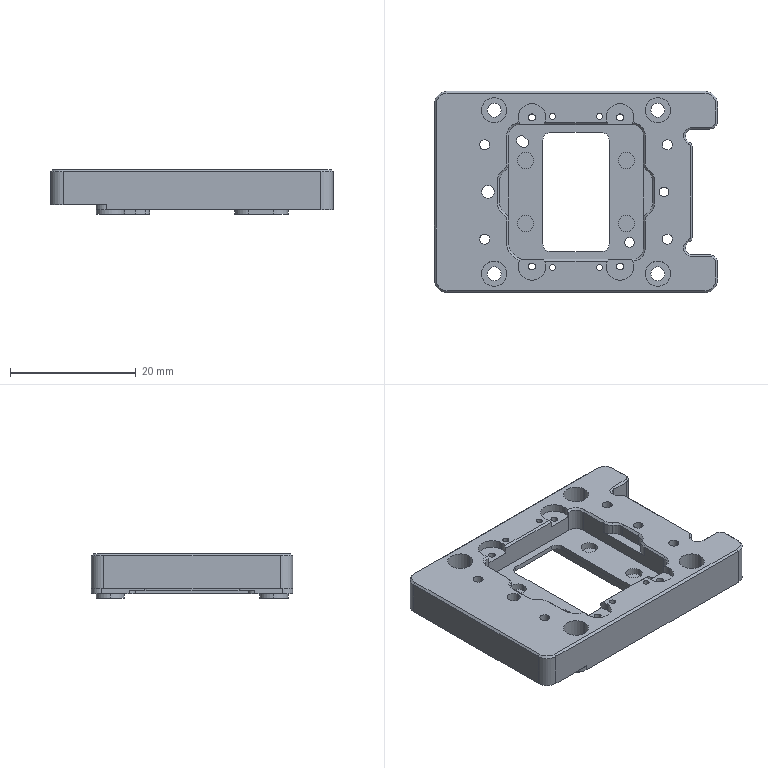NC program | NX | posted with a generic post | part box 45 x 32 x 7.05 mm
Lines 1284 to 2424 of 5787:
(CAVITY_MILL , TOOL : D3)
N2518 T17 M6
N2520 G54
N2522 G17 G0 G90 X-5.414 Y8.674 S9500 M3
N2524 G43 Z30. H17
N2526 Z0.75
N2528 G94 G1 Z-0.25 F1100.
N2530 G3 X-5.887 Y9.474 R1.
N2532 G2 X-6.394 Y11.499 R1.498
N2534 G3 X-7.606 Y11.5 R-0.7
N2536 G2 X-8.12 Y9.472 R1.505
N2538 G3 X-8.594 Y8.592 R1.
N2540 G1 X-8.563 Y7.553
N2542 Z0.75
N2544 G0 Z30.
N2546 X-5.938 Y8.753
N2548 Z0.75
N2550 G1 Z-0.25
N2552 X-7.156 Y9.453
N2554 G3 X-8.156 Y9.451 R1.
N2556 G2 X-9. Y9.25 R1.505
N2558 G3 X-9.25 Y9. R0.25
N2560 G1 Y7.912
N2562 G3 X-8.75 Y7.046 R1.
N2564 G1 X-8.65 Y6.988
N2566 Z0.75
N2568 G0 Z30.
N2570 X-5.417 Y8.6
N2572 Z0.5
N2574 G1 Z-0.5
N2576 G3 X-5.899 Y9.416 R1.
N2578 G2 X-6.403 Y11.484 R1.5
N2580 G3 X-7.7 Y11.835 R-0.7
N2582 X-7.581 Y11.458 R0.701
N2584 G2 X-8.101 Y9.416 R1.5
N2586 G3 X-7.722 Y9.742 R0.5
N2588 G1 X-7.646 Y8.644
N2590 Z0.5
N2592 G0 Z30.
N2594 X-5.417 Y8.6
N2596 Z0.25
N2598 G1 Z-0.75
N2600 G3 X-5.899 Y9.416 R1.
N2602 G2 X-6.403 Y11.484 R1.5
N2604 G3 X-7.7 Y11.835 R-0.7
N2606 X-7.581 Y11.458 R0.701
N2608 G2 X-8.101 Y9.416 R1.5
N2610 G3 X-7.722 Y9.742 R0.5
N2612 G1 X-7.646 Y8.644
N2614 Z0.25
N2616 G0 Z30.
N2618 X-5.417 Y8.6
N2620 Z0.
N2622 G1 Z-1.
N2624 G3 X-5.899 Y9.416 R1.
N2626 G2 X-6.528 Y11.229 R1.5
N2628 X-6.388 Y11.51 R1.501
N2630 G3 X-7.597 Y11.484 R-0.7
N2632 G2 X-8.101 Y9.416 R1.5
N2634 G3 X-7.722 Y9.742 R0.5
N2636 G1 X-7.213 Y8.766
N2638 Z0.
N2640 G0 X-5.417 Y8.6 Z-0.25
N2642 G1 Z-1.25
N2644 G3 X-5.899 Y9.416 R1.
N2646 G2 X-6.528 Y11.229 R1.5
N2648 X-6.388 Y11.51 R1.501
N2650 G3 X-7.7 Y11.835 R-0.7
N2652 X-7.592 Y11.477 R0.7
N2654 G2 X-8.101 Y9.416 R1.5
N2656 G3 X-7.722 Y9.742 R0.5
N2658 G1 X-7.213 Y8.766
N2660 Z-0.25
N2662 G0 Z30.
N2664 X-1.255 Y7.4
N2666 Z-3.113
N2668 G1 Z-4.113
N2670 X-1.312 Y7.5
N2672 G3 X-2.178 Y8. R1.
N2674 G1 X-3.75
N2676 Y6.428
N2678 G3 X-3.25 Y5.562 R1.
N2680 G1 X-3.15 Y5.505
N2682 Z-3.113
N2684 G0 X-1.255 Y7.4 Z-3.375
N2686 G1 Z-4.375
N2688 X-1.312 Y7.5
N2690 G3 X-2.178 Y8. R1.
N2692 G1 X-3.75
N2694 Y6.428
N2696 G3 X-3.25 Y5.562 R1.
N2698 G1 X-3.15 Y5.505
N2700 Z-3.375
N2702 G0 X-1.256 Y7.4 Z-3.638
N2704 G1 Z-4.638
N2706 X-1.314 Y7.5
N2708 G3 X-2.18 Y8. R1.
N2710 G1 X-3.75
N2712 Y6.43
N2714 G3 X-3.25 Y5.564 R1.
N2716 G1 X-3.15 Y5.506
N2718 Z-3.638
N2720 G0 X-1.256 Y7.4 Z-3.9
N2722 G1 Z-4.9
N2724 X-1.314 Y7.5
N2726 G3 X-2.18 Y8. R1.
N2728 G1 X-3.75
N2730 Y6.43
N2732 G3 X-3.25 Y5.564 R1.
N2734 G1 X-3.15 Y5.506
N2736 Z-3.9
N2738 G0 X-1.256 Y7.4 Z-4.169
N2740 G1 Z-5.169
N2742 X-1.314 Y7.5
N2744 G3 X-2.18 Y8. R1.
N2746 G1 X-3.75
N2748 Y6.43
N2750 G3 X-3.25 Y5.564 R1.
N2752 G1 X-3.15 Y5.506
N2754 Z-4.169
N2756 G0 X-1.256 Y7.4 Z-4.438
N2758 G1 Z-5.438
N2760 X-1.314 Y7.5
N2762 G3 X-2.18 Y8. R1.
N2764 G1 X-3.75
N2766 Y6.43
N2768 G3 X-3.25 Y5.564 R1.
N2770 G1 X-3.15 Y5.506
N2772 Z-4.438
N2774 G0 X-1.256 Y7.4 Z-4.706
N2776 G1 Z-5.706
N2778 X-1.314 Y7.5
N2780 G3 X-2.18 Y8. R1.
N2782 G1 X-3.75
N2784 Y6.43
N2786 G3 X-3.25 Y5.564 R1.
N2788 G1 X-3.15 Y5.506
N2790 Z-4.706
N2792 G0 X-1.256 Y7.4 Z-4.975
N2794 G1 Z-5.975
N2796 X-1.314 Y7.5
N2798 G3 X-2.18 Y8. R1.
N2800 G1 X-3.75
N2802 Y6.43
N2804 G3 X-3.25 Y5.564 R1.
N2806 G1 X-3.15 Y5.506
N2808 Z-4.975
N2810 G0 X-1.256 Y7.4 Z-5.244
N2812 G1 Z-6.244
N2814 X-1.314 Y7.5
N2816 G3 X-2.18 Y8. R1.
N2818 G1 X-3.75
N2820 Y6.43
N2822 G3 X-3.25 Y5.564 R1.
N2824 G1 X-3.15 Y5.506
N2826 Z-5.244
N2828 G0 X-1.256 Y7.4 Z-5.513
N2830 G1 Z-6.513
N2832 X-1.314 Y7.5
N2834 G3 X-2.18 Y8. R1.
N2836 G1 X-3.75
N2838 Y6.43
N2840 G3 X-3.25 Y5.564 R1.
N2842 G1 X-3.15 Y5.506
N2844 Z-5.513
N2846 G0 X-1.256 Y7.4 Z-5.781
N2848 G1 Z-6.781
N2850 X-1.314 Y7.5
N2852 G3 X-2.18 Y8. R1.
N2854 G1 X-3.75
N2856 Y6.43
N2858 G3 X-3.25 Y5.564 R1.
N2860 G1 X-3.15 Y5.506
N2862 Z-5.781
N2864 G0 X-1.256 Y7.4 Z-6.05
N2866 G1 Z-7.05
N2868 X-1.314 Y7.5
N2870 G3 X-2.18 Y8. R1.
N2872 G1 X-3.75
N2874 Y6.43
N2876 G3 X-3.25 Y5.564 R1.
N2878 G1 X-3.15 Y5.506
N2880 Z-6.05
N2882 G0 Z30.
N2884 X-5.649 Y8.6
N2886 Z0.5
N2888 G1 Z-0.5
N2890 X-7.111 Y9.421
N2892 G3 X-8.111 Y9.41 R1.
N2894 G2 X-8.876 Y9.2 R1.5
N2896 G1 X-9.
N2898 G3 X-9.2 Y9. R0.2
N2900 G1 Y7.868
N2902 G3 X-8.7 Y7.002 R1.
N2904 G1 X-8.6 Y6.945
N2906 Z0.5
N2908 G0 Z30.
N2910 X-5.649 Y8.6
N2912 Z0.25
N2914 G1 Z-0.75
N2916 X-7.111 Y9.421
N2918 G3 X-8.111 Y9.41 R1.
N2920 G2 X-8.876 Y9.2 R1.5
N2922 G1 X-9.
N2924 G3 X-9.2 Y9. R0.2
N2926 G1 Y7.868
N2928 G3 X-8.7 Y7.002 R1.
N2930 G1 X-8.6 Y6.945
N2932 Z0.25
N2934 G0 Z30.
N2936 X-5.649 Y8.6
N2938 Z0.
N2940 G1 Z-1.
N2942 X-7.111 Y9.421
N2944 G3 X-8.111 Y9.41 R1.
N2946 G2 X-8.876 Y9.2 R1.5
N2948 G1 X-9.
N2950 G3 X-9.2 Y9. R0.2
N2952 G1 Y7.868
N2954 G3 X-8.7 Y7.002 R1.
N2956 G1 X-8.6 Y6.945
N2958 Z0.
N2960 G0 X-5.649 Y8.6 Z-0.25
N2962 G1 Z-1.25
N2964 X-7.111 Y9.421
N2966 G3 X-8.111 Y9.41 R1.
N2968 G2 X-8.876 Y9.2 R1.5
N2970 G1 X-9.
N2972 G3 X-9.2 Y9. R0.2
N2974 G1 Y7.868
N2976 G3 X-8.7 Y7.002 R1.
N2978 G1 X-8.6 Y6.945
N2980 Z-0.25
N2982 G0 X-6.705 Y8.6 Z-0.5
N2984 G1 Z-1.5
N2986 X-6.762 Y8.7
N2988 G3 X-7.628 Y9.2 R1.
N2990 G1 X-9.
N2992 G3 X-9.2 Y9. R0.2
N2994 G1 Y7.628
N2996 G3 X-8.7 Y6.762 R1.
N2998 G1 X-8.6 Y6.705
N3000 Z-0.5
N3002 G0 X-6.705 Y8.6 Z-0.75
N3004 G1 Z-1.75
N3006 X-6.762 Y8.7
N3008 G3 X-7.628 Y9.2 R1.
N3010 G1 X-9.
N3012 G3 X-9.2 Y9. R0.2
N3014 G1 Y7.628
N3016 G3 X-8.7 Y6.762 R1.
N3018 G1 X-8.6 Y6.705
N3020 Z-0.75
N3022 G0 X-6.705 Y8.6 Z-1.
N3024 G1 Z-2.
N3026 X-6.762 Y8.7
N3028 G3 X-7.628 Y9.2 R1.
N3030 G1 X-9.
N3032 G3 X-9.2 Y9. R0.2
N3034 G1 Y7.628
N3036 G3 X-8.7 Y6.762 R1.
N3038 G1 X-8.6 Y6.705
N3040 Z-1.
N3042 G0 X-6.705 Y8.6 Z-1.25
N3044 G1 Z-2.25
N3046 X-6.762 Y8.7
N3048 G3 X-7.628 Y9.2 R1.
N3050 G1 X-9.
N3052 G3 X-9.2 Y9. R0.2
N3054 G1 Y7.628
N3056 G3 X-8.7 Y6.762 R1.
N3058 G1 X-8.6 Y6.705
N3060 Z-1.25
N3062 G0 X-6.705 Y8.6 Z-1.5
N3064 G1 Z-2.5
N3066 X-6.762 Y8.7
N3068 G3 X-7.628 Y9.2 R1.
N3070 G1 X-9.
N3072 G3 X-9.2 Y9. R0.2
N3074 G1 Y7.628
N3076 G3 X-8.7 Y6.762 R1.
N3078 G1 X-8.6 Y6.705
N3080 Z-1.5
N3082 G0 X-6.705 Y8.6 Z-1.75
N3084 G1 Z-2.75
N3086 X-6.762 Y8.7
N3088 G3 X-7.628 Y9.2 R1.
N3090 G1 X-9.
N3092 G3 X-9.2 Y9. R0.2
N3094 G1 Y7.628
N3096 G3 X-8.7 Y6.762 R1.
N3098 G1 X-8.6 Y6.705
N3100 Z-1.75
N3102 G0 X-6.705 Y8.6 Z-2.
N3104 G1 Z-3.
N3106 X-6.762 Y8.7
N3108 G3 X-7.628 Y9.2 R1.
N3110 G1 X-9.
N3112 G3 X-9.2 Y9. R0.2
N3114 G1 Y7.628
N3116 G3 X-8.7 Y6.762 R1.
N3118 G1 X-8.6 Y6.705
N3120 Z-2.
N3122 G0 X-6.705 Y8.6 Z-2.283
N3124 G1 Z-3.283
N3126 X-6.762 Y8.7
N3128 G3 X-7.628 Y9.2 R1.
N3130 G1 X-9.
N3132 G3 X-9.2 Y9. R0.2
N3134 G1 Y7.628
N3136 G3 X-8.7 Y6.762 R1.
N3138 G1 X-8.6 Y6.705
N3140 Z-2.283
N3142 G0 X-6.705 Y8.6 Z-2.567
N3144 G1 Z-3.567
N3146 X-6.762 Y8.7
N3148 G3 X-7.628 Y9.2 R1.
N3150 G1 X-9.
N3152 G3 X-9.2 Y9. R0.2
N3154 G1 Y7.628
N3156 G3 X-8.7 Y6.762 R1.
N3158 G1 X-8.6 Y6.705
N3160 Z-2.567
N3162 G0 X-6.705 Y8.6 Z-2.85
N3164 G1 Z-3.85
N3166 X-6.762 Y8.7
N3168 G3 X-7.628 Y9.2 R1.
N3170 G1 X-9.
N3172 G3 X-9.2 Y9. R0.2
N3174 G1 Y7.628
N3176 G3 X-8.7 Y6.762 R1.
N3178 G1 X-8.6 Y6.705
N3180 Z-2.85
N3182 G0 Z30.
N3184 X-9.203 Y2.649
N3186 Z0.75
N3188 G1 Z-0.25
N3190 G3 X-10.166 Y2.381 R1.
N3192 G2 X-10.621 Y1.996 R3.2
N3194 G3 X-10.75 Y1.75 R0.3
N3196 G1 Y1.108
N3198 G3 X-10.25 Y0.242 R1.
N3200 G1 X-10.15 Y0.185
N3202 Z0.75
N3204 G0 Z30.
N3206 X-9.158 Y2.625
N3208 Z0.5
N3210 G1 X-9.16 Y2.626 Z-0.5
N3212 G3 X-10.122 Y2.354 R1.
N3214 G2 X-10.593 Y1.955 R3.25
N3216 G3 X-10.7 Y1.75 R0.25
N3218 G1 Y1.087
N3220 G3 X-10.2 Y0.221 R1.
N3222 G1 X-10.1 Y0.163
N3224 Z0.5
N3226 G0 Z30.
N3228 X-9.158 Y2.625
N3230 Z0.25
N3232 G1 X-9.16 Y2.626 Z-0.75
N3234 G3 X-10.122 Y2.354 R1.
N3236 G2 X-10.593 Y1.955 R3.25
N3238 G3 X-10.7 Y1.75 R0.25
N3240 G1 Y1.087
N3242 G3 X-10.2 Y0.221 R1.
N3244 G1 X-10.1 Y0.163
N3246 Z0.25
N3248 G0 Z30.
N3250 X-9.158 Y2.625
N3252 Z0.
N3254 G1 X-9.16 Y2.626 Z-1.
N3256 G3 X-10.122 Y2.354 R1.
N3258 G2 X-10.593 Y1.955 R3.25
N3260 G3 X-10.7 Y1.75 R0.25
N3262 G1 Y1.087
N3264 G3 X-10.2 Y0.221 R1.
N3266 G1 X-10.1 Y0.163
N3268 Z0.
N3270 G0 X-9.158 Y2.625 Z-0.25
N3272 G1 X-9.16 Y2.626 Z-1.25
N3274 G3 X-10.122 Y2.354 R1.
N3276 G2 X-10.593 Y1.955 R3.25
N3278 G3 X-10.7 Y1.75 R0.25
N3280 G1 Y1.087
N3282 G3 X-10.2 Y0.221 R1.
N3284 G1 X-10.1 Y0.163
N3286 Z-0.25
N3288 G0 X-9.158 Y2.625 Z-0.5
N3290 G1 X-9.16 Y2.626 Z-1.5
N3292 G3 X-10.122 Y2.354 R1.
N3294 G2 X-10.593 Y1.955 R3.25
N3296 G3 X-10.7 Y1.75 R0.25
N3298 G1 Y1.087
N3300 G3 X-10.2 Y0.221 R1.
N3302 G1 X-10.1 Y0.163
N3304 Z-0.5
N3306 G0 X-9.158 Y2.625 Z-0.75
N3308 G1 X-9.16 Y2.626 Z-1.75
N3310 G3 X-10.122 Y2.354 R1.
N3312 G2 X-10.593 Y1.955 R3.25
N3314 G3 X-10.7 Y1.75 R0.25
N3316 G1 Y1.087
N3318 G3 X-10.2 Y0.221 R1.
N3320 G1 X-10.1 Y0.163
N3322 Z-0.75
N3324 G0 X-9.158 Y2.625 Z-1.
N3326 G1 X-9.16 Y2.626 Z-2.
N3328 G3 X-10.122 Y2.354 R1.
N3330 G2 X-10.593 Y1.955 R3.25
N3332 G3 X-10.7 Y1.75 R0.25
N3334 G1 Y1.087
N3336 G3 X-10.2 Y0.221 R1.
N3338 G1 X-10.1 Y0.163
N3340 Z-1.
N3342 G0 Z30.
N3344 X-10.15 Y-0.185
N3346 Z0.75
N3348 G1 Z-0.25
N3350 X-10.25 Y-0.242
N3352 G3 X-10.75 Y-1.108 R1.
N3354 G1 Y-1.75
N3356 G3 X-10.621 Y-1.996 R0.3
N3358 G2 X-10.166 Y-2.381 R3.2
N3360 G3 X-9.203 Y-2.649 R1.
N3362 G1 Z0.75
N3364 G0 Z30.
N3366 X-10.1 Y-0.163
N3368 Z0.5
N3370 G1 Z-0.5
N3372 X-10.2 Y-0.221
N3374 G3 X-10.7 Y-1.087 R1.
N3376 G1 Y-1.75
N3378 G3 X-10.593 Y-1.955 R0.25
N3380 G2 X-10.122 Y-2.354 R3.25
N3382 G3 X-9.158 Y-2.625 R1.
N3384 G1 Z0.5
N3386 G0 Z30.
N3388 X-10.1 Y-0.163
N3390 Z0.25
N3392 G1 Z-0.75
N3394 X-10.2 Y-0.221
N3396 G3 X-10.7 Y-1.087 R1.
N3398 G1 Y-1.75
N3400 G3 X-10.593 Y-1.955 R0.25
N3402 G2 X-10.122 Y-2.354 R3.25
N3404 G3 X-9.158 Y-2.625 R1.
N3406 G1 Z0.25
N3408 G0 Z30.
N3410 X-10.1 Y-0.163
N3412 Z0.
N3414 G1 Z-1.
N3416 X-10.2 Y-0.221
N3418 G3 X-10.7 Y-1.087 R1.
N3420 G1 Y-1.75
N3422 G3 X-10.593 Y-1.955 R0.25
N3424 G2 X-10.122 Y-2.354 R3.25
N3426 G3 X-9.158 Y-2.625 R1.
N3428 G1 Z0.
N3430 G0 X-10.1 Y-0.163 Z-0.25
N3432 G1 Z-1.25
N3434 X-10.2 Y-0.221
N3436 G3 X-10.7 Y-1.087 R1.
N3438 G1 Y-1.75
N3440 G3 X-10.593 Y-1.955 R0.25
N3442 G2 X-10.122 Y-2.354 R3.25
N3444 G3 X-9.158 Y-2.625 R1.
N3446 G1 Z-0.25
N3448 G0 X-10.1 Y-0.163 Z-0.5
N3450 G1 Z-1.5
N3452 X-10.2 Y-0.221
N3454 G3 X-10.7 Y-1.087 R1.
N3456 G1 Y-1.75
N3458 G3 X-10.593 Y-1.955 R0.25
N3460 G2 X-10.122 Y-2.354 R3.25
N3462 G3 X-9.158 Y-2.625 R1.
N3464 G1 Z-0.5
N3466 G0 X-10.1 Y-0.163 Z-0.75
N3468 G1 Z-1.75
N3470 X-10.2 Y-0.221
N3472 G3 X-10.7 Y-1.087 R1.
N3474 G1 Y-1.75
N3476 G3 X-10.593 Y-1.955 R0.25
N3478 G2 X-10.122 Y-2.354 R3.25
N3480 G3 X-9.158 Y-2.625 R1.
N3482 G1 Z-0.75
N3484 G0 X-10.1 Y-0.163 Z-1.
N3486 G1 Z-2.
N3488 X-10.2 Y-0.221
N3490 G3 X-10.7 Y-1.087 R1.
N3492 G1 Y-1.75
N3494 G3 X-10.593 Y-1.955 R0.25
N3496 G2 X-10.122 Y-2.354 R3.25
N3498 G3 X-9.158 Y-2.625 R1.
N3500 G1 Z-1.
N3502 G0 Z30.
N3504 X-8.65 Y-6.866
N3506 Z0.75
N3508 G1 Z-0.25
N3510 X-8.75 Y-6.923
N3512 G3 X-9.25 Y-7.789 R1.
N3514 G1 Y-8.379
N3516 X-9.259 Y-8.486
N3518 X-9.177 Y-8.555
N3520 X-8.76 Y-8.972
N3522 G3 X-7.794 Y-9.231 R1.
N3524 G1 X-5.904 Y-8.725
N3526 Z0.75
N3528 G0 Z30.
N3530 X-8.6 Y-6.845
N3532 Z0.5
N3534 G1 Z-0.5
N3536 X-8.7 Y-6.903
N3538 G3 X-9.2 Y-7.769 R1.
N3540 G1 Y-8.379
N3542 X-9.212 Y-8.467
N3544 X-9.141 Y-8.52
N3546 X-8.71 Y-8.951
N3548 G3 X-8.227 Y-9.081 R0.5
N3550 G1 X-7.036 Y-8.762
N3552 Z0.5
N3554 G0 Z30.
N3556 X-8.6 Y-6.845
N3558 Z0.25
N3560 G1 Z-0.75
N3562 X-8.7 Y-6.903
N3564 G3 X-9.2 Y-7.769 R1.
N3566 G1 Y-8.379
N3568 X-9.212 Y-8.467
N3570 X-9.141 Y-8.52
N3572 X-8.71 Y-8.951
N3574 G3 X-8.227 Y-9.081 R0.5
N3576 G1 X-7.036 Y-8.762
N3578 Z0.25
N3580 G0 Z30.
N3582 X-8.6 Y-6.845
N3584 Z0.
N3586 G1 Z-1.
N3588 X-8.7 Y-6.903
N3590 G3 X-9.2 Y-7.769 R1.
N3592 G1 Y-8.379
N3594 X-9.212 Y-8.467
N3596 X-9.141 Y-8.52
N3598 X-8.71 Y-8.951
N3600 G3 X-8.227 Y-9.081 R0.5
N3602 G1 X-7.036 Y-8.762
N3604 Z0.
N3606 G0 X-8.6 Y-6.845 Z-0.25
N3608 G1 Z-1.25
N3610 X-8.7 Y-6.903
N3612 G3 X-9.2 Y-7.769 R1.
N3614 G1 Y-8.379
N3616 X-9.212 Y-8.467
N3618 X-9.141 Y-8.52
N3620 X-8.71 Y-8.951
N3622 G3 X-8.227 Y-9.081 R0.5
N3624 G1 X-7.036 Y-8.762
N3626 Z-0.25
N3628 G0 Z30.
N3630 X-8.485 Y-7.499
N3632 Z0.75
N3634 G1 Z-0.25
N3636 X-8.526 Y-8.528
N3638 G3 X-8.061 Y-9.414 R1.
N3640 G2 X-7.584 Y-11.464 R1.498
N3642 G3 X-6.394 Y-11.499 R-0.7
N3644 G2 X-5.852 Y-9.453 R1.498
N3646 G3 X-5.358 Y-8.666 R1.
N3648 G1 Z0.75
N3650 G0 Z30.
N3652 X-8.497 Y-7.423
N3654 Z0.5
N3656 G1 Z-0.5
N3658 X-8.526 Y-8.48
N3660 G3 X-8.05 Y-9.36 R1.
N3662 G2 X-7.584 Y-11.464 R1.5
N3664 G3 X-6.3 Y-11.844 R-0.7
N3666 X-6.419 Y-11.458 R0.701
N3668 G2 X-5.867 Y-9.396 R1.5
N3670 G3 X-5.365 Y-8.614 R1.
N3672 G1 Z0.5
N3674 G0 Z30.
N3676 X-8.497 Y-7.423
N3678 Z0.25
N3680 G1 Z-0.75
N3682 X-8.526 Y-8.48
N3684 G3 X-8.05 Y-9.36 R1.
N3686 G2 X-7.584 Y-11.464 R1.5
N3688 G3 X-6.3 Y-11.844 R-0.7
N3690 X-6.419 Y-11.458 R0.701
N3692 G2 X-5.867 Y-9.396 R1.5
N3694 G3 X-5.365 Y-8.614 R1.
N3696 G1 Z0.25
N3698 G0 Z30.
N3700 X-8.497 Y-7.423
N3702 Z0.
N3704 G1 Z-1.
N3706 X-8.526 Y-8.48
N3708 G3 X-8.05 Y-9.36 R1.
N3710 G2 X-7.584 Y-11.464 R1.5
N3712 G3 X-6.3 Y-11.844 R-0.7
N3714 X-6.406 Y-11.479 R0.7
N3716 G2 X-5.867 Y-9.396 R1.5
N3718 G3 X-5.365 Y-8.614 R1.
N3720 G1 Z0.
N3722 G0 X-8.497 Y-7.423 Z-0.25
N3724 G1 Z-1.25
N3726 X-8.526 Y-8.48
N3728 G3 X-8.05 Y-9.36 R1.
N3730 G2 X-7.584 Y-11.464 R1.5
N3732 G3 X-6.3 Y-11.844 R-0.7
N3734 X-6.411 Y-11.472 R0.7
N3736 G2 X-5.867 Y-9.396 R1.5
N3738 G3 X-5.365 Y-8.614 R1.
N3740 G1 Z-0.25
N3742 G0 X-8.6 Y-6.705 Z-0.5
N3744 G1 Z-1.5
N3746 X-8.7 Y-6.762
N3748 G3 X-9.2 Y-7.628 R1.
N3750 G1 Y-8.379
N3752 X-9.212 Y-8.467
N3754 X-9.141 Y-8.52
N3756 X-8.52 Y-9.141
N3758 X-8.467 Y-9.212
N3760 X-8.379 Y-9.2
N3762 X-7.628
N3764 G3 X-6.762 Y-8.7 R1.
N3766 G1 X-6.705 Y-8.6
N3768 Z-0.5
N3770 G0 X-8.6 Y-6.705 Z-0.75
N3772 G1 Z-1.75
N3774 X-8.7 Y-6.762
N3776 G3 X-9.2 Y-7.628 R1.
N3778 G1 Y-8.379
N3780 X-9.212 Y-8.467
N3782 X-9.141 Y-8.52
N3784 X-8.52 Y-9.141
N3786 X-8.467 Y-9.212
N3788 X-8.379 Y-9.2
N3790 X-7.628
N3792 G3 X-6.762 Y-8.7 R1.
N3794 G1 X-6.705 Y-8.6
N3796 Z-0.75
N3798 G0 X-8.6 Y-6.705 Z-1.
N3800 G1 Z-2.
N3802 X-8.7 Y-6.762
N3804 G3 X-9.2 Y-7.628 R1.
N3806 G1 Y-8.379
N3808 X-9.212 Y-8.467
N3810 X-9.141 Y-8.52
N3812 X-8.52 Y-9.141
N3814 X-8.467 Y-9.212
N3816 X-8.379 Y-9.2
N3818 X-7.628
N3820 G3 X-6.762 Y-8.7 R1.
N3822 G1 X-6.705 Y-8.6
N3824 Z-1.
N3826 G0 X-8.6 Y-6.705 Z-1.25
N3828 G1 Z-2.25
N3830 X-8.7 Y-6.762
N3832 G3 X-9.2 Y-7.628 R1.
N3834 G1 Y-8.379
N3836 X-9.212 Y-8.467
N3838 X-9.141 Y-8.52
N3840 X-8.52 Y-9.141
N3842 X-8.467 Y-9.212
N3844 X-8.379 Y-9.2
N3846 X-7.628
N3848 G3 X-6.762 Y-8.7 R1.
N3850 G1 X-6.705 Y-8.6
N3852 Z-1.25
N3854 G0 X-8.6 Y-6.705 Z-1.5
N3856 G1 Z-2.5
N3858 X-8.7 Y-6.762
N3860 G3 X-9.2 Y-7.628 R1.
N3862 G1 Y-8.379
N3864 X-9.212 Y-8.467
N3866 X-9.141 Y-8.52
N3868 X-8.52 Y-9.141
N3870 X-8.467 Y-9.212
N3872 X-8.379 Y-9.2
N3874 X-7.628
N3876 G3 X-6.762 Y-8.7 R1.
N3878 G1 X-6.705 Y-8.6
N3880 Z-1.5
N3882 G0 X-8.6 Y-6.705 Z-1.75
N3884 G1 Z-2.75
N3886 X-8.7 Y-6.762
N3888 G3 X-9.2 Y-7.628 R1.
N3890 G1 Y-8.379
N3892 X-9.212 Y-8.467
N3894 X-9.141 Y-8.52
N3896 X-8.52 Y-9.141
N3898 X-8.467 Y-9.212
N3900 X-8.379 Y-9.2
N3902 X-7.628
N3904 G3 X-6.762 Y-8.7 R1.
N3906 G1 X-6.705 Y-8.6
N3908 Z-1.75
N3910 G0 X-8.6 Y-6.705 Z-2.
N3912 G1 Z-3.
N3914 X-8.7 Y-6.762
N3916 G3 X-9.2 Y-7.628 R1.
N3918 G1 Y-8.379
N3920 X-9.212 Y-8.467
N3922 X-9.141 Y-8.52
N3924 X-8.52 Y-9.141
N3926 X-8.467 Y-9.212
N3928 X-8.379 Y-9.2
N3930 X-7.628
N3932 G3 X-6.762 Y-8.7 R1.
N3934 G1 X-6.705 Y-8.6
N3936 Z-2.
N3938 G0 X-8.6 Y-6.705 Z-2.283
N3940 G1 Z-3.283
N3942 X-8.7 Y-6.762
N3944 G3 X-9.2 Y-7.628 R1.
N3946 G1 Y-8.379
N3948 X-9.212 Y-8.467
N3950 X-9.141 Y-8.52
N3952 X-8.52 Y-9.141
N3954 X-8.467 Y-9.212
N3956 X-8.379 Y-9.2
N3958 X-7.628
N3960 G3 X-6.762 Y-8.7 R1.
N3962 G1 X-6.705 Y-8.6
N3964 Z-2.283
N3966 G0 X-8.6 Y-6.705 Z-2.567
N3968 G1 Z-3.567
N3970 X-8.7 Y-6.762
N3972 G3 X-9.2 Y-7.628 R1.
N3974 G1 Y-8.379
N3976 X-9.212 Y-8.467
N3978 X-9.141 Y-8.52
N3980 X-8.52 Y-9.141
N3982 X-8.467 Y-9.212
N3984 X-8.379 Y-9.2
N3986 X-7.628
N3988 G3 X-6.762 Y-8.7 R1.
N3990 G1 X-6.705 Y-8.6
N3992 Z-2.567
N3994 G0 X-8.6 Y-6.705 Z-2.85
N3996 G1 Z-3.85
N3998 X-8.7 Y-6.762
N4000 G3 X-9.2 Y-7.628 R1.
N4002 G1 Y-8.379
N4004 X-9.212 Y-8.467
N4006 X-9.141 Y-8.52
N4008 X-8.52 Y-9.141
N4010 X-8.467 Y-9.212
N4012 X-8.379 Y-9.2
N4014 X-7.628
N4016 G3 X-6.762 Y-8.7 R1.
N4018 G1 X-6.705 Y-8.6
N4020 Z-2.85
N4022 G0 Z30.
N4024 X-3.15 Y-5.505
N4026 Z-3.113
N4028 G1 Z-4.113
N4030 X-3.25 Y-5.562
N4032 G3 X-3.75 Y-6.428 R1.
N4034 G1 Y-8.
N4036 X-2.178
N4038 G3 X-1.312 Y-7.5 R1.
N4040 G1 X-1.255 Y-7.4
N4042 Z-3.113
N4044 G0 X-3.15 Y-5.505 Z-3.375
N4046 G1 Z-4.375
N4048 X-3.25 Y-5.562
N4050 G3 X-3.75 Y-6.428 R1.
N4052 G1 Y-8.
N4054 X-2.178
N4056 G3 X-1.312 Y-7.5 R1.
N4058 G1 X-1.255 Y-7.4
N4060 Z-3.375
N4062 G0 X-3.15 Y-5.506 Z-3.638
N4064 G1 Z-4.638
N4066 X-3.25 Y-5.564
N4068 G3 X-3.75 Y-6.43 R1.
N4070 G1 Y-8.
N4072 X-2.18
N4074 G3 X-1.314 Y-7.5 R1.
N4076 G1 X-1.256 Y-7.4
N4078 Z-3.638
N4080 G0 X-3.15 Y-5.506 Z-3.9
N4082 G1 Z-4.9
N4084 X-3.25 Y-5.564
N4086 G3 X-3.75 Y-6.43 R1.
N4088 G1 Y-8.
N4090 X-2.18
N4092 G3 X-1.314 Y-7.5 R1.
N4094 G1 X-1.256 Y-7.4
N4096 Z-3.9
N4098 G0 X-3.15 Y-5.506 Z-4.169
N4100 G1 Z-5.169
N4102 X-3.25 Y-5.564
N4104 G3 X-3.75 Y-6.43 R1.
N4106 G1 Y-8.
N4108 X-2.18
N4110 G3 X-1.314 Y-7.5 R1.
N4112 G1 X-1.256 Y-7.4
N4114 Z-4.169
N4116 G0 X-3.15 Y-5.506 Z-4.438
N4118 G1 Z-5.438
N4120 X-3.25 Y-5.564
N4122 G3 X-3.75 Y-6.43 R1.
N4124 G1 Y-8.
N4126 X-2.18
N4128 G3 X-1.314 Y-7.5 R1.
N4130 G1 X-1.256 Y-7.4
N4132 Z-4.438
N4134 G0 X-3.15 Y-5.506 Z-4.706
N4136 G1 Z-5.706
N4138 X-3.25 Y-5.564
N4140 G3 X-3.75 Y-6.43 R1.
N4142 G1 Y-8.
N4144 X-2.18
N4146 G3 X-1.314 Y-7.5 R1.
N4148 G1 X-1.256 Y-7.4
N4150 Z-4.706
N4152 G0 X-3.15 Y-5.506 Z-4.975
N4154 G1 Z-5.975
N4156 X-3.25 Y-5.564
N4158 G3 X-3.75 Y-6.43 R1.
N4160 G1 Y-8.
N4162 X-2.18
N4164 G3 X-1.314 Y-7.5 R1.
N4166 G1 X-1.256 Y-7.4
N4168 Z-4.975
N4170 G0 X-3.15 Y-5.506 Z-5.244
N4172 G1 Z-6.244
N4174 X-3.25 Y-5.564
N4176 G3 X-3.75 Y-6.43 R1.
N4178 G1 Y-8.
N4180 X-2.18
N4182 G3 X-1.314 Y-7.5 R1.
N4184 G1 X-1.256 Y-7.4
N4186 Z-5.244
N4188 G0 X-3.15 Y-5.506 Z-5.513
N4190 G1 Z-6.513
N4192 X-3.25 Y-5.564
N4194 G3 X-3.75 Y-6.43 R1.
N4196 G1 Y-8.
N4198 X-2.18
N4200 G3 X-1.314 Y-7.5 R1.
N4202 G1 X-1.256 Y-7.4
N4204 Z-5.513
N4206 G0 X-3.15 Y-5.506 Z-5.781
N4208 G1 Z-6.781
N4210 X-3.25 Y-5.564
N4212 G3 X-3.75 Y-6.43 R1.
N4214 G1 Y-8.
N4216 X-2.18
N4218 G3 X-1.314 Y-7.5 R1.
N4220 G1 X-1.256 Y-7.4
N4222 Z-5.781
N4224 G0 X-3.15 Y-5.506 Z-6.05
N4226 G1 Z-7.05
N4228 X-3.25 Y-5.564
N4230 G3 X-3.75 Y-6.43 R1.
N4232 G1 Y-8.
N4234 X-2.18
N4236 G3 X-1.314 Y-7.5 R1.
N4238 G1 X-1.256 Y-7.4
N4240 Z-6.05
N4242 G0 Z30.
N4244 X5.415 Y-8.674
N4246 Z0.75
N4248 G1 Z-0.25
N4250 G3 X5.887 Y-9.475 R1.
N4252 G2 X6.394 Y-11.499 R1.498
N4254 G3 X7.606 Y-11.5 R-0.7
N4256 G2 X8.12 Y-9.473 R1.505
N4258 G3 X8.593 Y-8.592 R1.
N4260 G1 X8.561 Y-7.554
N4262 Z0.75
N4264 G0 Z30.
N4266 X5.94 Y-8.754
N4268 Z0.75
N4270 G1 Z-0.25
N4272 X7.156 Y-9.453
N4274 G3 X8.156 Y-9.451 R1.
N4276 G2 X9. Y-9.25 R1.505
N4278 G3 X9.25 Y-9. R0.25
N4280 G1 Y-7.912
N4282 G3 X8.75 Y-7.046 R1.
N4284 G1 X8.65 Y-6.988
N4286 Z0.75
N4288 G0 Z30.
N4290 X5.417 Y-8.6
N4292 Z0.5
N4294 G1 Z-0.5
N4296 G3 X5.899 Y-9.416 R1.
N4298 G2 X6.403 Y-11.484 R1.5
N4300 G3 X7.7 Y-11.835 R-0.7
N4302 X7.581 Y-11.458 R0.701
N4304 G2 X8.101 Y-9.416 R1.5
N4306 G3 X7.722 Y-9.742 R0.5
N4308 G1 X7.213 Y-8.766
N4310 Z0.5
N4312 G0 Z30.
N4314 X5.417 Y-8.6
N4316 Z0.25
N4318 G1 Z-0.75
N4320 G3 X5.899 Y-9.416 R1.
N4322 G2 X6.403 Y-11.484 R1.5
N4324 G3 X7.7 Y-11.835 R-0.7
N4326 X7.581 Y-11.458 R0.701
N4328 G2 X8.101 Y-9.416 R1.5
N4330 G3 X7.722 Y-9.742 R0.5
N4332 G1 X7.213 Y-8.766
N4334 Z0.25
N4336 G0 Z30.
N4338 X5.417 Y-8.6
N4340 Z0.
N4342 G1 Z-1.
N4344 G3 X5.899 Y-9.416 R1.
N4346 G2 X6.388 Y-11.51 R1.501
N4348 G3 X7.597 Y-11.484 R-0.7
N4350 G2 X8.101 Y-9.416 R1.5
N4352 G3 X7.722 Y-9.742 R0.5
N4354 G1 X7.213 Y-8.766
N4356 Z0.
N4358 G0 X5.417 Y-8.6 Z-0.25
N4360 G1 Z-1.25
N4362 G3 X5.899 Y-9.416 R1.
N4364 G2 X6.388 Y-11.51 R1.501
N4366 G3 X7.7 Y-11.835 R-0.7
N4368 X7.593 Y-11.478 R0.7
N4370 G2 X8.101 Y-9.416 R1.5
N4372 G3 X7.722 Y-9.742 R0.5
N4374 G1 X7.213 Y-8.766
N4376 Z-0.25
N4378 G0 Z30.
N4380 X1.255 Y-7.4
N4382 Z-3.113
N4384 G1 Z-4.113
N4386 X1.312 Y-7.5
N4388 G3 X2.178 Y-8. R1.
N4390 G1 X3.75
N4392 Y-6.428
N4394 G3 X3.25 Y-5.562 R1.
N4396 G1 X3.15 Y-5.505
N4398 Z-3.113
N4400 G0 X1.255 Y-7.4 Z-3.375
N4402 G1 Z-4.375
N4404 X1.312 Y-7.5
N4406 G3 X2.178 Y-8. R1.
N4408 G1 X3.75
N4410 Y-6.428
N4412 G3 X3.25 Y-5.562 R1.
N4414 G1 X3.15 Y-5.505
N4416 Z-3.375
N4418 G0 X1.256 Y-7.4 Z-3.638
N4420 G1 Z-4.638
N4422 X1.314 Y-7.5
N4424 G3 X2.18 Y-8. R1.
N4426 G1 X3.75
N4428 Y-6.43
N4430 G3 X3.25 Y-5.564 R1.
N4432 G1 X3.15 Y-5.506
N4434 Z-3.638
N4436 G0 X1.256 Y-7.4 Z-3.9
N4438 G1 Z-4.9
N4440 X1.314 Y-7.5
N4442 G3 X2.18 Y-8. R1.
N4444 G1 X3.75
N4446 Y-6.43
N4448 G3 X3.25 Y-5.564 R1.
N4450 G1 X3.15 Y-5.506
N4452 Z-3.9
N4454 G0 X1.256 Y-7.4 Z-4.169
N4456 G1 Z-5.169
N4458 X1.314 Y-7.5
N4460 G3 X2.18 Y-8. R1.
N4462 G1 X3.75
N4464 Y-6.43
N4466 G3 X3.25 Y-5.564 R1.
N4468 G1 X3.15 Y-5.506
N4470 Z-4.169
N4472 G0 X1.256 Y-7.4 Z-4.438
N4474 G1 Z-5.438
N4476 X1.314 Y-7.5
N4478 G3 X2.18 Y-8. R1.
N4480 G1 X3.75
N4482 Y-6.43
N4484 G3 X3.25 Y-5.564 R1.
N4486 G1 X3.15 Y-5.506
N4488 Z-4.438
N4490 G0 X1.256 Y-7.4 Z-4.706
N4492 G1 Z-5.706
N4494 X1.314 Y-7.5
N4496 G3 X2.18 Y-8. R1.
N4498 G1 X3.75
N4500 Y-6.43
N4502 G3 X3.25 Y-5.564 R1.
N4504 G1 X3.15 Y-5.506
N4506 Z-4.706
N4508 G0 X1.256 Y-7.4 Z-4.975
N4510 G1 Z-5.975
N4512 X1.314 Y-7.5
N4514 G3 X2.18 Y-8. R1.
N4516 G1 X3.75
N4518 Y-6.43
N4520 G3 X3.25 Y-5.564 R1.
N4522 G1 X3.15 Y-5.506
N4524 Z-4.975
N4526 G0 X1.256 Y-7.4 Z-5.244
N4528 G1 Z-6.244
N4530 X1.314 Y-7.5
N4532 G3 X2.18 Y-8. R1.
N4534 G1 X3.75
N4536 Y-6.43
N4538 G3 X3.25 Y-5.564 R1.
N4540 G1 X3.15 Y-5.506
N4542 Z-5.244
N4544 G0 X1.256 Y-7.4 Z-5.513
N4546 G1 Z-6.513
N4548 X1.314 Y-7.5
N4550 G3 X2.18 Y-8. R1.
N4552 G1 X3.75
N4554 Y-6.43
N4556 G3 X3.25 Y-5.564 R1.
N4558 G1 X3.15 Y-5.506
N4560 Z-5.513
N4562 G0 X1.256 Y-7.4 Z-5.781
N4564 G1 Z-6.781
N4566 X1.314 Y-7.5
N4568 G3 X2.18 Y-8. R1.
N4570 G1 X3.75
N4572 Y-6.43
N4574 G3 X3.25 Y-5.564 R1.
N4576 G1 X3.15 Y-5.506
N4578 Z-5.781
N4580 G0 X1.256 Y-7.4 Z-6.05
N4582 G1 Z-7.05
N4584 X1.314 Y-7.5
N4586 G3 X2.18 Y-8. R1.
N4588 G1 X3.75
N4590 Y-6.43
N4592 G3 X3.25 Y-5.564 R1.
N4594 G1 X3.15 Y-5.506
N4596 Z-6.05
N4598 G0 Z30.
N4600 X5.649 Y-8.6
N4602 Z0.5
N4604 G1 Z-0.5
N4606 X7.111 Y-9.421
N4608 G3 X8.111 Y-9.41 R1.
N4610 G2 X8.876 Y-9.2 R1.5
N4612 G1 X9.
N4614 G3 X9.2 Y-9. R0.2
N4616 G1 Y-7.868
N4618 G3 X8.7 Y-7.002 R1.
N4620 G1 X8.6 Y-6.945
N4622 Z0.5
N4624 G0 Z30.
N4626 X5.649 Y-8.6
N4628 Z0.25
N4630 G1 Z-0.75
N4632 X7.111 Y-9.421
N4634 G3 X8.111 Y-9.41 R1.
N4636 G2 X8.876 Y-9.2 R1.5
N4638 G1 X9.
N4640 G3 X9.2 Y-9. R0.2
N4642 G1 Y-7.868
N4644 G3 X8.7 Y-7.002 R1.
N4646 G1 X8.6 Y-6.945
N4648 Z0.25
N4650 G0 Z30.
N4652 X5.649 Y-8.6
N4654 Z0.
N4656 G1 Z-1.
N4658 X7.111 Y-9.421
N4660 G3 X8.111 Y-9.41 R1.
N4662 G2 X8.876 Y-9.2 R1.5
N4664 G1 X9.
N4666 G3 X9.2 Y-9. R0.2
N4668 G1 Y-7.868
N4670 G3 X8.7 Y-7.002 R1.
N4672 G1 X8.6 Y-6.945
N4674 Z0.
N4676 G0 X5.649 Y-8.6 Z-0.25
N4678 G1 Z-1.25
N4680 X7.111 Y-9.421
N4682 G3 X8.111 Y-9.41 R1.
N4684 G2 X8.876 Y-9.2 R1.5
N4686 G1 X9.
N4688 G3 X9.2 Y-9. R0.2
N4690 G1 Y-7.868
N4692 G3 X8.7 Y-7.002 R1.
N4694 G1 X8.6 Y-6.945
N4696 Z-0.25
N4698 G0 X6.705 Y-8.6 Z-0.5
N4700 G1 Z-1.5
N4702 X6.762 Y-8.7
N4704 G3 X7.628 Y-9.2 R1.
N4706 G1 X9.
N4708 G3 X9.2 Y-9. R0.2
N4710 G1 Y-7.628
N4712 G3 X8.7 Y-6.762 R1.
N4714 G1 X8.6 Y-6.705
N4716 Z-0.5
N4718 G0 X6.705 Y-8.6 Z-0.75
N4720 G1 Z-1.75
N4722 X6.762 Y-8.7
N4724 G3 X7.628 Y-9.2 R1.
N4726 G1 X9.
N4728 G3 X9.2 Y-9. R0.2
N4730 G1 Y-7.628
N4732 G3 X8.7 Y-6.762 R1.
N4734 G1 X8.6 Y-6.705
N4736 Z-0.75
N4738 G0 X6.705 Y-8.6 Z-1.
N4740 G1 Z-2.
N4742 X6.762 Y-8.7
N4744 G3 X7.628 Y-9.2 R1.
N4746 G1 X9.
N4748 G3 X9.2 Y-9. R0.2
N4750 G1 Y-7.628
N4752 G3 X8.7 Y-6.762 R1.
N4754 G1 X8.6 Y-6.705
N4756 Z-1.
N4758 G0 X6.705 Y-8.6 Z-1.25
N4760 G1 Z-2.25
N4762 X6.762 Y-8.7
N4764 G3 X7.628 Y-9.2 R1.
N4766 G1 X9.
N4768 G3 X9.2 Y-9. R0.2
N4770 G1 Y-7.628
N4772 G3 X8.7 Y-6.762 R1.
N4774 G1 X8.6 Y-6.705
N4776 Z-1.25
N4778 G0 X6.705 Y-8.6 Z-1.5
N4780 G1 Z-2.5
N4782 X6.762 Y-8.7
N4784 G3 X7.628 Y-9.2 R1.
N4786 G1 X9.
N4788 G3 X9.2 Y-9. R0.2
N4790 G1 Y-7.628
N4792 G3 X8.7 Y-6.762 R1.